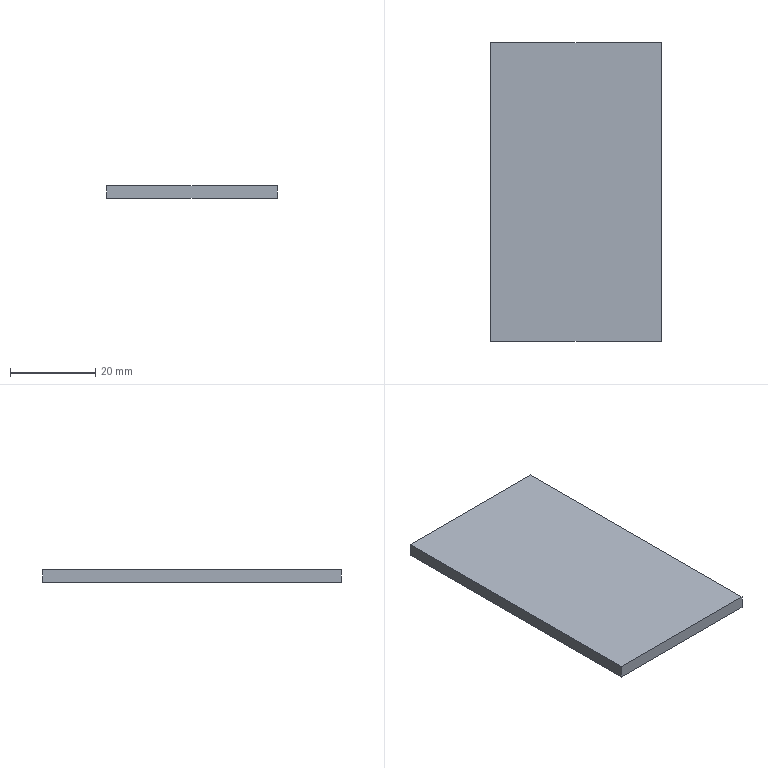Part | SolidWorks | features Extrusion 1 | 1 solid | 6 faces | box 40 x 70 x 3 mm | volume 8400 mm3 | plane 6
STEP:
#1=CARTESIAN_POINT('',(0.,70.,0.));
#2=VERTEX_POINT('',#1);
#3=CARTESIAN_POINT('',(0.,0.,0.));
#4=VERTEX_POINT('',#3);
#5=CARTESIAN_POINT('',(0.,70.,0.));
#6=DIRECTION('',(0.,-1.,0.));
#7=VECTOR('',#6,1000.);
#8=LINE('',#5,#7);
#9=EDGE_CURVE('',#2,#4,#8,.T.);
#10=ORIENTED_EDGE('',*,*,#9,.T.);
#11=CARTESIAN_POINT('',(0.,0.,3.));
#12=VERTEX_POINT('',#11);
#13=CARTESIAN_POINT('',(0.,0.,3.));
#14=DIRECTION('',(0.,0.,-1.));
#15=VECTOR('',#14,1000.);
#16=LINE('',#13,#15);
#17=EDGE_CURVE('',#12,#4,#16,.T.);
#18=ORIENTED_EDGE('',*,*,#17,.F.);
#19=CARTESIAN_POINT('',(0.,70.,3.));
#20=VERTEX_POINT('',#19);
#21=CARTESIAN_POINT('',(0.,70.,3.));
#22=DIRECTION('',(0.,-1.,0.));
#23=VECTOR('',#22,1000.);
#24=LINE('',#21,#23);
#25=EDGE_CURVE('',#20,#12,#24,.T.);
#26=ORIENTED_EDGE('',*,*,#25,.F.);
#27=CARTESIAN_POINT('',(0.,70.,3.));
#28=DIRECTION('',(0.,0.,-1.));
#29=VECTOR('',#28,1000.);
#30=LINE('',#27,#29);
#31=EDGE_CURVE('',#20,#2,#30,.T.);
#32=ORIENTED_EDGE('',*,*,#31,.T.);
#33=EDGE_LOOP('',(#10,#18,#26,#32));
#34=FACE_OUTER_BOUND('',#33,.T.);
#35=CARTESIAN_POINT('',(0.,70.,3.));
#36=DIRECTION('',(1.,0.,0.));
#37=DIRECTION('',(0.,0.,-1.));
#38=AXIS2_PLACEMENT_3D('',#35,#36,#37);
#39=PLANE('',#38);
#40=ADVANCED_FACE('',(#34),#39,.F.);
#41=CARTESIAN_POINT('',(40.,0.,0.));
#42=VERTEX_POINT('',#41);
#43=CARTESIAN_POINT('',(0.,0.,0.));
#44=DIRECTION('',(1.,0.,0.));
#45=VECTOR('',#44,1000.);
#46=LINE('',#43,#45);
#47=EDGE_CURVE('',#4,#42,#46,.T.);
#48=ORIENTED_EDGE('',*,*,#47,.T.);
#49=CARTESIAN_POINT('',(40.,0.,3.));
#50=VERTEX_POINT('',#49);
#51=CARTESIAN_POINT('',(40.,0.,3.));
#52=DIRECTION('',(0.,0.,-1.));
#53=VECTOR('',#52,1000.);
#54=LINE('',#51,#53);
#55=EDGE_CURVE('',#50,#42,#54,.T.);
#56=ORIENTED_EDGE('',*,*,#55,.F.);
#57=CARTESIAN_POINT('',(0.,0.,3.));
#58=DIRECTION('',(1.,0.,0.));
#59=VECTOR('',#58,1000.);
#60=LINE('',#57,#59);
#61=EDGE_CURVE('',#12,#50,#60,.T.);
#62=ORIENTED_EDGE('',*,*,#61,.F.);
#63=ORIENTED_EDGE('',*,*,#17,.T.);
#64=EDGE_LOOP('',(#48,#56,#62,#63));
#65=FACE_OUTER_BOUND('',#64,.T.);
#66=CARTESIAN_POINT('',(0.,0.,3.));
#67=DIRECTION('',(0.,1.,0.));
#68=DIRECTION('',(0.,0.,1.));
#69=AXIS2_PLACEMENT_3D('',#66,#67,#68);
#70=PLANE('',#69);
#71=ADVANCED_FACE('',(#65),#70,.F.);
#72=CARTESIAN_POINT('',(40.,70.,0.));
#73=VERTEX_POINT('',#72);
#74=CARTESIAN_POINT('',(40.,0.,0.));
#75=DIRECTION('',(0.,1.,0.));
#76=VECTOR('',#75,1000.);
#77=LINE('',#74,#76);
#78=EDGE_CURVE('',#42,#73,#77,.T.);
#79=ORIENTED_EDGE('',*,*,#78,.T.);
#80=CARTESIAN_POINT('',(40.,70.,3.));
#81=VERTEX_POINT('',#80);
#82=CARTESIAN_POINT('',(40.,70.,3.));
#83=DIRECTION('',(0.,0.,-1.));
#84=VECTOR('',#83,1000.);
#85=LINE('',#82,#84);
#86=EDGE_CURVE('',#81,#73,#85,.T.);
#87=ORIENTED_EDGE('',*,*,#86,.F.);
#88=CARTESIAN_POINT('',(40.,0.,3.));
#89=DIRECTION('',(0.,1.,0.));
#90=VECTOR('',#89,1000.);
#91=LINE('',#88,#90);
#92=EDGE_CURVE('',#50,#81,#91,.T.);
#93=ORIENTED_EDGE('',*,*,#92,.F.);
#94=ORIENTED_EDGE('',*,*,#55,.T.);
#95=EDGE_LOOP('',(#79,#87,#93,#94));
#96=FACE_OUTER_BOUND('',#95,.T.);
#97=CARTESIAN_POINT('',(40.,0.,3.));
#98=DIRECTION('',(-1.,0.,0.));
#99=DIRECTION('',(0.,0.,1.));
#100=AXIS2_PLACEMENT_3D('',#97,#98,#99);
#101=PLANE('',#100);
#102=ADVANCED_FACE('',(#96),#101,.F.);
#103=CARTESIAN_POINT('',(40.,70.,0.));
#104=DIRECTION('',(-1.,0.,0.));
#105=VECTOR('',#104,1000.);
#106=LINE('',#103,#105);
#107=EDGE_CURVE('',#73,#2,#106,.T.);
#108=ORIENTED_EDGE('',*,*,#107,.T.);
#109=ORIENTED_EDGE('',*,*,#31,.F.);
#110=CARTESIAN_POINT('',(40.,70.,3.));
#111=DIRECTION('',(-1.,0.,0.));
#112=VECTOR('',#111,1000.);
#113=LINE('',#110,#112);
#114=EDGE_CURVE('',#81,#20,#113,.T.);
#115=ORIENTED_EDGE('',*,*,#114,.F.);
#116=ORIENTED_EDGE('',*,*,#86,.T.);
#117=EDGE_LOOP('',(#108,#109,#115,#116));
#118=FACE_OUTER_BOUND('',#117,.T.);
#119=CARTESIAN_POINT('',(40.,70.,3.));
#120=DIRECTION('',(0.,-1.,0.));
#121=DIRECTION('',(0.,0.,-1.));
#122=AXIS2_PLACEMENT_3D('',#119,#120,#121);
#123=PLANE('',#122);
#124=ADVANCED_FACE('',(#118),#123,.F.);
#125=ORIENTED_EDGE('',*,*,#25,.T.);
#126=ORIENTED_EDGE('',*,*,#61,.T.);
#127=ORIENTED_EDGE('',*,*,#92,.T.);
#128=ORIENTED_EDGE('',*,*,#114,.T.);
#129=EDGE_LOOP('',(#125,#126,#127,#128));
#130=FACE_OUTER_BOUND('',#129,.T.);
#131=CARTESIAN_POINT('',(0.,0.,3.));
#132=DIRECTION('',(0.,0.,1.));
#133=DIRECTION('',(1.,0.,0.));
#134=AXIS2_PLACEMENT_3D('',#131,#132,#133);
#135=PLANE('',#134);
#136=ADVANCED_FACE('',(#130),#135,.T.);
#137=ORIENTED_EDGE('',*,*,#9,.F.);
#138=ORIENTED_EDGE('',*,*,#107,.F.);
#139=ORIENTED_EDGE('',*,*,#78,.F.);
#140=ORIENTED_EDGE('',*,*,#47,.F.);
#141=EDGE_LOOP('',(#137,#138,#139,#140));
#142=FACE_OUTER_BOUND('',#141,.T.);
#143=CARTESIAN_POINT('',(0.,0.,0.));
#144=DIRECTION('',(0.,0.,1.));
#145=DIRECTION('',(1.,0.,0.));
#146=AXIS2_PLACEMENT_3D('',#143,#144,#145);
#147=PLANE('',#146);
#148=ADVANCED_FACE('',(#142),#147,.F.);
#149=CLOSED_SHELL('',(#40,#71,#102,#124,#136,#148));
#150=MANIFOLD_SOLID_BREP('',#149);
#151=CARTESIAN_POINT('',(0.,0.,0.));
#152=DIRECTION('',(0.,0.,1.));
#153=DIRECTION('',(1.,0.,0.));
#154=AXIS2_PLACEMENT_3D('',#151,#152,#153);
#155=(LENGTH_UNIT()NAMED_UNIT(*)SI_UNIT(.MILLI.,.METRE.));
#156=UNCERTAINTY_MEASURE_WITH_UNIT(LENGTH_MEASURE(0.00001),#155,'','');
#157=(NAMED_UNIT(*)PLANE_ANGLE_UNIT()SI_UNIT($,.RADIAN.));
#158=(NAMED_UNIT(*)SI_UNIT($,.STERADIAN.)SOLID_ANGLE_UNIT());
#159=(GEOMETRIC_REPRESENTATION_CONTEXT(3)GLOBAL_UNCERTAINTY_ASSIGNED_CONTEXT((#156))GLOBAL_UNIT_ASSIGNED_CONTEXT((#155,#157,#158))REPRESENTATION_CONTEXT('',''));
#160=ADVANCED_BREP_SHAPE_REPRESENTATION('',(#150,#154),#159);